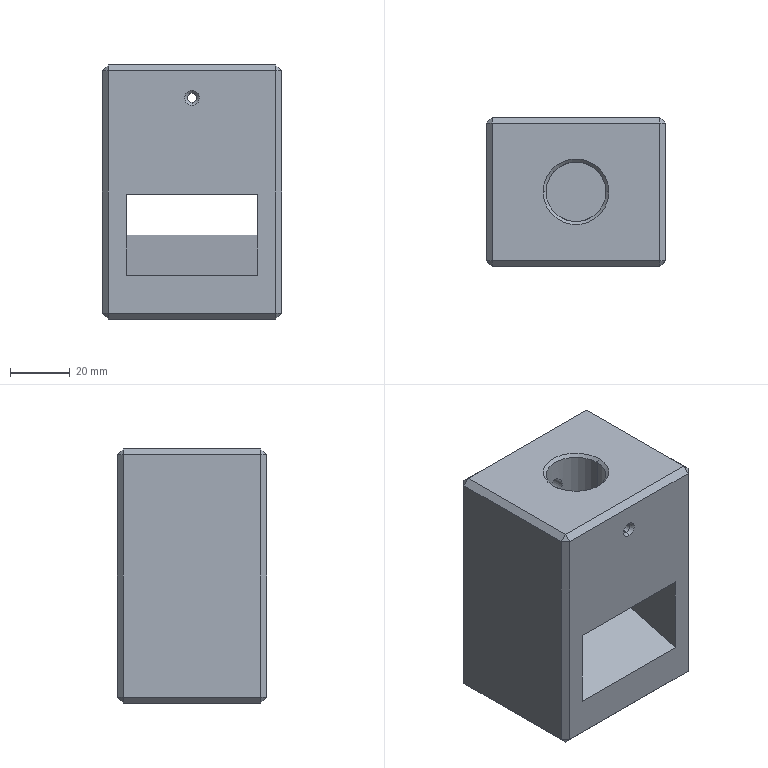Part | STEP file | Gaveta - Torre - 5 cav | 1 solid | 47 faces | box 60 x 50 x 85 mm | volume 186270 mm3 | plane 31 | cone 8 | cylinder 8 | commonest cylinder face diameters 6 x4 3 x2 20 x2